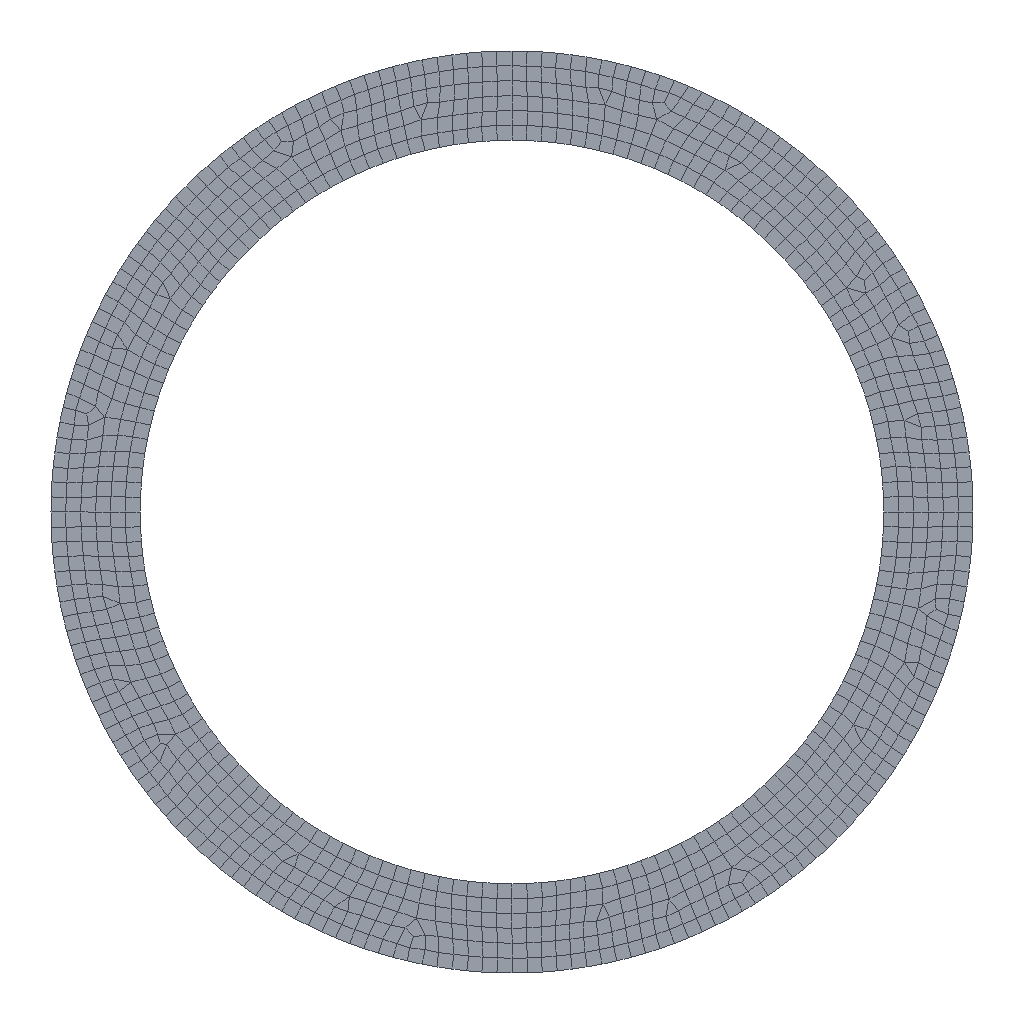Simulation study | ansys workbench
Set-up summary:
category,name,step,type,value,unit,region
solver,ansys_workbench
units,mm-N-s-tonne (MPa),,stated,"/units,MPA"
analysis,LS1,,static
load_step,LS1,LS1,static,nsubst=1; time=1
mesh,nodes,,,3513
mesh,elements,,,1443
element_type,PLANE183,,,1059
element_type,SURF153,,,384
material,?,,E,34500,tonne s^-2 mm^-1
material,?,,nu,0.2
material,?,,density,2.5e-09,tonne mm^-3
load,Define Pressure Using Surface Effect Elements,LS1,pressure,3,,SURF153 #3
load,Define Pressure Using Surface Effect Elements,LS1,pressure,3,,SURF153 #4
load,Define Pressure Using Surface Effect Elements,LS1,pressure,4,,SURF153 #5
load,Define Pressure Using Surface Effect Elements,LS1,pressure,4,,SURF153 #6
bc,Constant Zero Displacement X,model,fixed,[dofs=UX],,_DISPZEROUX
bc,Constant Zero Displacement Y,model,fixed,[dofs=UY],,_DISPZEROUY
named_set,_DISPZEROUX,,node,1
named_set,_DISPZEROUY,,node,1
Ansys APDL input file, long lists of numbers shortened:
/batch
/config,noeldb,1     ! force off writing results to database
*get,_wallstrt,active,,time,wall
! ANSYS input file written by Workbench version 2021 R1
! File used for geometry attach:
/title,____--____ (C5)
! ****** Begin Custom Load Command Snippet ******
/COM, ACT Extensions:
/COM,     LSDYNA, 2021.1
/COM,
! ****** End   Custom Load Command Snippet ******
*DIM,_wb_ProjectScratch_dir,string,248
_wb_ProjectScratch_dir(1) = ''
*DIM,_wb_SolverFiles_dir,string,248
_wb_SolverFiles_dir(1) = ''
*DIM,_wb_userfiles_dir,string,248
_wb_userfiles_dir(1) = ''
/com,--- Data in consistent NMM units. See Solving Units in the help system for more information.
/units,MPA
/nopr
/wb,file,start              !  signify a WB generated input file
/prep7
! Turn off shape checking because checks already performed inside WB mesher.
! See help system for more information.
SHPP,OFF,,NOWARN
/nolist
etcon,set             ! allow ANSYS to choose best KEYOP's for 180x elements, resets any applicable keyopt to MAPDL defaults
/com,*********** Nodes for the whole assembly ***********
nblock,3,,3864
(1i9,3e20.9e3)
        1     0.000000000E+00     3.100000000E+03     0.000000000E+00
! (3512 more lines like these left out)
-1
/wb,elem,start            !  set before creation of elements
/com,*********** Elements for Body 1 "_______-FreeParts|NONE" ***********
et,1,183
keyo,1,3,3
eblock,19,solid,,1059
(19i9)
        1        1        1        1        0        0        0        0        8        0        1      716      715      804      804     2627     2629      804     2632
! (1058 more lines like these left out)
-1
/wb,elem,end               !  done creating elements
/com,*********** Send User Defined Coordinate System(s) ***********
csys,0
toffst,273.15,  ! Temperature offset from absolute zero
/com,*********** Set Reference Temperature ***********
tref,22.
/wb,mat,start              !  starting to send materials
/com,*********** Send Materials ***********
MP,DENS,1,2.5e-09,	! tonne mm^-3
MP,EX,1,34500,	! tonne s^-2 mm^-1
MP,NUXY,1,0.2,
/wb,mat,end                !  done sending materials
/com,*********** Send Sheet Properties ***********
r,1,100.
!************************* Model Summary ********************
!_______-FreeParts|NONE,	支护,	matid,	1
!************************* End Model Summary ********************
! get the diagonal of the bounding box. Needed later for other things
*get,_xmin,node,,mnloc,x
*get,_ymin,node,,mnloc,y
*get,_zmin,node,,mnloc,z
*get,_xmax,node,,mxloc,x
*get,_ymax,node,,mxloc,y
*get,_zmax,node,,mxloc,z
_ASMDIAG=(_xmax-_xmin)*(_xmax-_xmin)+(_ymax-_ymin)*(_ymax-_ymin)+(_zmax-_zmin)*(_zmax-_zmin)
_ASMDIAG=SQRT(_ASMDIAG)
/wb,contact,start          !  starting to send contact
/wb,contact,end            !  done creating contacts
/golist
/wb,load,start             !  starting to send loads
/com,******* Constant Zero Displacement X *******
CMBLOCK,_DISPZEROUX,NODE,        1
(8i10)
       326
cmsel,s,_DISPZEROUX
d,all,ux,0
nsel,all
/com,******* Constant Zero Displacement Y *******
CMBLOCK,_DISPZEROUY,NODE,        1
(8i10)
       326
cmsel,s,_DISPZEROUY
d,all,uy,0
nsel,all
/com,*********** Create Elastic Support ***********
et,2,153
keyop,2,3,10        ! get plane stress option and thickness from underlying element
eblock,10,,,192
(15i9)
     1060        2        2        2        0      204      227     1656
! (191 more lines like these left out)
-1
esel,s,type,,2
r,2,,,,5.e-002
esel,all
/com,*********** Define Pressure Using Surface Effect Elements ***********
et,3,153
keyop,3,3,10        ! get plane stress option and thickness from underlying element
eblock,10,,,48
(15i9)
     1252        3        3        3        0        2       25     1231
! (47 more lines like these left out)
-1
esel,s,type,,3
keyop,3,7,0                ! Use deformed area for application of load
esel,all
/com,*********** Define Pressure Using Surface Effect Elements ***********
et,4,153
keyop,4,3,10        ! get plane stress option and thickness from underlying element
eblock,10,,,48
(15i9)
     1300        4        4        4        0      302      373     1862
! (47 more lines like these left out)
-1
esel,s,type,,4
keyop,4,7,0                ! Use deformed area for application of load
esel,all
/com,*********** Define Pressure Using Surface Effect Elements ***********
et,5,153
keyop,5,3,10        ! get plane stress option and thickness from underlying element
eblock,10,,,48
(15i9)
     1348        5        5        5        0      204      227     1656
! (47 more lines like these left out)
-1
esel,s,type,,5
keyop,5,7,0                ! Use deformed area for application of load
esel,all
/com,*********** Define Pressure Using Surface Effect Elements ***********
et,6,153
keyop,6,3,10        ! get plane stress option and thickness from underlying element
eblock,10,,,48
(15i9)
     1396        6        6        6        0      129      128     1497
! (47 more lines like these left out)
-1
esel,s,type,,6
keyop,6,7,0                ! Use deformed area for application of load
esel,all
esel,all
/gst,on,on
fini
*get,_numnode,node,0,count
*get,_numelem,elem,0,count
*get, _MAXELEMNUM, elem, 0, NUM, MAX
*get, _MAXNODENUM, node, 0, NUM, MAX
*get, _MAXELEMTYPE, etyp, 0, NUM, MAX
*get, _MAXREALCONST, real, 0, NUM, MAX
/go
/wb,load,end               !  done creating loads
/com,--- Number of total nodes = %_numnode%
/com,--- Number of contact elements = 384
/com,--- Number of spring elements = 0
/com,--- Number of bearing elements = 0
/com,--- Number of solid elements = 1059
/com,--- Number of condensed parts = 0
/com,--- Number of total elements = %_numelem%
*get,_wallbsol,active,,time,wall
/com,****************************************************************************
/com,*************************    SOLUTION       ********************************
/com,****************************************************************************
/solu
antype,0                   ! static analysis
_thickRatio=  0     ! Ratio of thick parts in the model
eqsl,sparse,,,,,1
cntr,print,1               ! print out contact info and also make no initial contact an error
dmpoption,emat,no             ! Don't combine emat file for DANSYS
dmpoption,esav,no             ! Don't combine esav file for DANSYS
nldiag,cont,iter           ! print out contact info each equilibrium iteration
rescontrol,,none                 ! Do not keep any restart files
/com,****************************************************
/com,******************* SOLVE FOR LS 1 OF 1 ****************
esel,s,type,,3
nsle
sf,all,pres,3.
esel,s,type,,4
nsle
sf,all,pres,3.
esel,s,type,,5
nsle
sf,all,pres,4.
esel,s,type,,6
nsle
sf,all,pres,4.
nsel,all
esel,all
acel,0.,9806.65
esel,all
/nopr
/gopr
/nolist
nsub,1,1,1
time,1.
outres,erase
outres,all,none
outres,nsol,all,
outres,rsol,all
outres,eangl,all
outres,etmp,all
outres,veng,all
outres,strs,all,
outres,epel,all,
outres,eppl,all,
outres,cont,all,
! *********** WB SOLVE COMMAND ***********
! check interactive state
*get,ANSINTER_,active,,int
*if,ANSINTER_,ne,0,then
/eof
*endif
solve
/com *************** Write FE CONNECTORS *********
CEWRITE,file,ce,,INTE
/com,****************************************************
/com,*************** FINISHED SOLVE FOR LS 1 *************
*get,_wallasol,active,,time,wall
/nopr
*get,_numnode,node,0,count
*get,_numelem,elem,0,count
*get, _MAXELEMNUM, elem, 0, NUM, MAX
*get, _MAXNODENUM, node, 0, NUM, MAX,,,INTERNAL
*get, _MAXELEMTYPE, etyp, 0, NUM, MAX
*get, _MAXREALCONST, real, 0, NUM, MAX
/gopr
/post1
xmlo,ENCODING,ISO-8859-1
xmlo,parm
/xml,parm,xml
fini
/gopr
*get,_walldone,active,,time,wall
_preptime=(_wallbsol-_wallstrt)*3600
_solvtime=(_wallasol-_wallbsol)*3600
_posttime=(_walldone-_wallasol)*3600
_totaltim=(_walldone-_wallstrt)*3600
*get,_dlbratio,active,0,solu,dlbr
*get,_combtime,active,0,solu,comb
/com,--- Total number of nodes = %_numnode%
/com,--- Total number of elements = %_numelem%
/com,--- Element load balance ratio = %_dlbratio%
/com,--- Time to combine distributed files = %_combtime%
/wb,file,end               ! done with WB generated input
Results summary:
result,analyses[0].index,,,1
result,analyses[0].system,,,SYS-2
result,analyses[0].deck,,,deck.dat
result,analyses[0].solve_status,,,completed
result,analyses[0].analysis_type,,,static
result,analyses[0].physics,,,mechanical
result,analyses[0].unit_system,,,"NMM: mm, ton, N, s, mV, mA, degC"
result,analyses[0].n_sets,,,1
result,analyses[0].load_steps[0].set,set=1,,1
result,analyses[0].load_steps[0].time_or_freq,set=1,,1
result,analyses[0].load_steps[0].max_displacement_magnitude,set=1,,5.747
result,analyses[0].load_steps[0].max_von_mises_nodal,set=1,,37.421
result,analyses[0].load_steps[0].reaction_force_sum_xyz[1],set=1,,1.6004e-06
result,analyses[0].load_steps[0].reaction_force_sum_xyz[2],set=1,,124338
result,analyses[0].load_steps[0].reaction_force_sum_xyz[3],set=1,,0
result,geometry_export[0][0],,,1.step
result,geometry_export[0][1],,,ok
result,geometry_export[0][2],,,1
result,geometry_export[1][0],,,2.step
result,geometry_export[1][1],,,ok
result,geometry_export[1][2],,,1